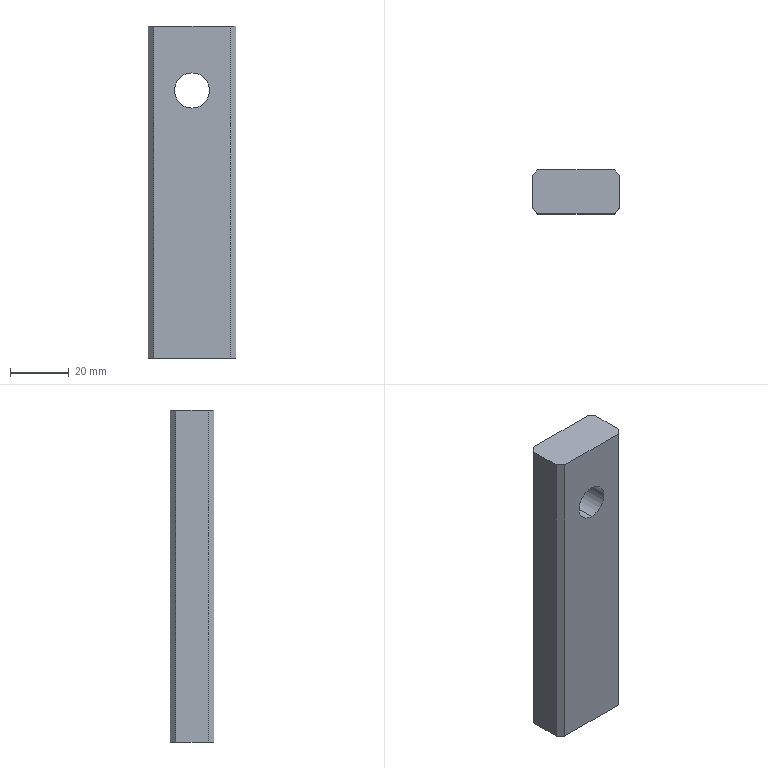Part | SolidWorks | features Cut 1, Extrusion 1, HoleWzd 1 | 1 solid | 18 faces | box 30 x 15 x 113.3 mm | volume 47736 mm3 | plane 10 | cone 4 | cylinder 4 | commonest cylinder face diameters 6.8 x2 12 x2
STEP:
#1=CARTESIAN_POINT('',(-96.6,33.5,0.625));
#2=VERTEX_POINT('',#1);
#3=CARTESIAN_POINT('',(-103.4,33.5,0.625));
#4=VERTEX_POINT('',#3);
#5=CARTESIAN_POINT('',(-100.,33.5,0.625));
#6=DIRECTION('',(0.,0.,-1.));
#7=DIRECTION('',(-1.,0.,0.));
#8=AXIS2_PLACEMENT_3D('',#5,#6,#7);
#9=CIRCLE('',#8,3.4);
#10=EDGE_CURVE('',#2,#4,#9,.T.);
#11=ORIENTED_EDGE('',*,*,#10,.F.);
#12=CARTESIAN_POINT('',(-95.975,33.5,0.));
#13=VERTEX_POINT('',#12);
#14=CARTESIAN_POINT('',(-95.975,33.5,0.));
#15=DIRECTION('',(0.7071,0.,-0.7071));
#16=VECTOR('',#15,1000.);
#17=LINE('',#14,#16);
#18=EDGE_CURVE('',#2,#13,#17,.T.);
#19=ORIENTED_EDGE('',*,*,#18,.T.);
#20=CARTESIAN_POINT('',(-104.025,33.5,0.));
#21=VERTEX_POINT('',#20);
#22=CARTESIAN_POINT('',(-100.,33.5,0.));
#23=DIRECTION('',(0.,0.,-1.));
#24=DIRECTION('',(-1.,0.,0.));
#25=AXIS2_PLACEMENT_3D('',#22,#23,#24);
#26=CIRCLE('',#25,4.025);
#27=EDGE_CURVE('',#13,#21,#26,.T.);
#28=ORIENTED_EDGE('',*,*,#27,.T.);
#29=CARTESIAN_POINT('',(-104.025,33.5,0.));
#30=DIRECTION('',(-0.7071,0.,-0.7071));
#31=VECTOR('',#30,1000.);
#32=LINE('',#29,#31);
#33=EDGE_CURVE('',#4,#21,#32,.T.);
#34=ORIENTED_EDGE('',*,*,#33,.F.);
#35=EDGE_LOOP('',(#11,#19,#28,#34));
#36=FACE_OUTER_BOUND('',#35,.T.);
#37=CARTESIAN_POINT('',(-100.,33.5,0.));
#38=DIRECTION('',(0.,0.,-1.));
#39=DIRECTION('',(-1.,0.,0.));
#40=AXIS2_PLACEMENT_3D('',#37,#38,#39);
#41=CONICAL_SURFACE('',#40,4.025,0.7854);
#42=ADVANCED_FACE('',(#36),#41,.F.);
#43=CARTESIAN_POINT('',(-96.6,33.5,17.));
#44=VERTEX_POINT('',#43);
#45=CARTESIAN_POINT('',(-103.4,33.5,17.));
#46=VERTEX_POINT('',#45);
#47=CARTESIAN_POINT('',(-100.,33.5,17.));
#48=DIRECTION('',(0.,0.,-1.));
#49=DIRECTION('',(-1.,0.,0.));
#50=AXIS2_PLACEMENT_3D('',#47,#48,#49);
#51=CIRCLE('',#50,3.4);
#52=EDGE_CURVE('',#44,#46,#51,.T.);
#53=ORIENTED_EDGE('',*,*,#52,.F.);
#54=CARTESIAN_POINT('',(-96.6,33.5,0.));
#55=DIRECTION('',(0.,0.,-1.));
#56=VECTOR('',#55,1000.);
#57=LINE('',#54,#56);
#58=EDGE_CURVE('',#44,#2,#57,.T.);
#59=ORIENTED_EDGE('',*,*,#58,.T.);
#60=ORIENTED_EDGE('',*,*,#10,.T.);
#61=CARTESIAN_POINT('',(-103.4,33.5,0.));
#62=DIRECTION('',(0.,0.,-1.));
#63=VECTOR('',#62,1000.);
#64=LINE('',#61,#63);
#65=EDGE_CURVE('',#46,#4,#64,.T.);
#66=ORIENTED_EDGE('',*,*,#65,.F.);
#67=EDGE_LOOP('',(#53,#59,#60,#66));
#68=FACE_OUTER_BOUND('',#67,.T.);
#69=CARTESIAN_POINT('',(-100.,33.5,0.));
#70=DIRECTION('',(0.,0.,-1.));
#71=DIRECTION('',(-1.,0.,0.));
#72=AXIS2_PLACEMENT_3D('',#69,#70,#71);
#73=CYLINDRICAL_SURFACE('',#72,3.4);
#74=ADVANCED_FACE('',(#68),#73,.F.);
#75=CARTESIAN_POINT('',(-100.,33.5,19.043));
#76=VERTEX_POINT('',#75);
#77=CARTESIAN_POINT('',(-103.4,33.5,17.));
#78=DIRECTION('',(-0.8572,0.,-0.515));
#79=VECTOR('',#78,1000.);
#80=LINE('',#77,#79);
#81=EDGE_CURVE('',#76,#46,#80,.T.);
#82=ORIENTED_EDGE('',*,*,#81,.F.);
#83=CARTESIAN_POINT('',(-96.6,33.5,17.));
#84=DIRECTION('',(0.8572,0.,-0.515));
#85=VECTOR('',#84,1000.);
#86=LINE('',#83,#85);
#87=EDGE_CURVE('',#76,#44,#86,.T.);
#88=ORIENTED_EDGE('',*,*,#87,.T.);
#89=ORIENTED_EDGE('',*,*,#52,.T.);
#90=EDGE_LOOP('',(#82,#88,#89));
#91=FACE_OUTER_BOUND('',#90,.T.);
#92=CARTESIAN_POINT('',(-100.,33.5,17.));
#93=DIRECTION('',(0.,0.,-1.));
#94=DIRECTION('',(-1.,0.,0.));
#95=AXIS2_PLACEMENT_3D('',#92,#93,#94);
#96=CONICAL_SURFACE('',#95,3.4,1.03);
#97=ADVANCED_FACE('',(#91),#96,.F.);
#98=CARTESIAN_POINT('',(-100.,41.,97.3));
#99=VERTEX_POINT('',#98);
#100=CARTESIAN_POINT('',(-100.,41.,85.3));
#101=VERTEX_POINT('',#100);
#102=CARTESIAN_POINT('',(-100.,41.,91.3));
#103=DIRECTION('',(0.,-1.,0.));
#104=DIRECTION('',(1.,0.,0.));
#105=AXIS2_PLACEMENT_3D('',#102,#103,#104);
#106=CIRCLE('',#105,6.);
#107=EDGE_CURVE('',#99,#101,#106,.T.);
#108=ORIENTED_EDGE('',*,*,#107,.F.);
#109=CARTESIAN_POINT('',(-100.,26.,97.3));
#110=VERTEX_POINT('',#109);
#111=CARTESIAN_POINT('',(-100.,136.,97.3));
#112=DIRECTION('',(0.,-1.,0.));
#113=VECTOR('',#112,1000.);
#114=LINE('',#111,#113);
#115=EDGE_CURVE('',#99,#110,#114,.T.);
#116=ORIENTED_EDGE('',*,*,#115,.T.);
#117=CARTESIAN_POINT('',(-100.,26.,85.3));
#118=VERTEX_POINT('',#117);
#119=CARTESIAN_POINT('',(-100.,26.,91.3));
#120=DIRECTION('',(0.,-1.,0.));
#121=DIRECTION('',(0.,0.,-1.));
#122=AXIS2_PLACEMENT_3D('',#119,#120,#121);
#123=CIRCLE('',#122,6.);
#124=EDGE_CURVE('',#110,#118,#123,.T.);
#125=ORIENTED_EDGE('',*,*,#124,.T.);
#126=CARTESIAN_POINT('',(-100.,136.,85.3));
#127=DIRECTION('',(0.,-1.,0.));
#128=VECTOR('',#127,1000.);
#129=LINE('',#126,#128);
#130=EDGE_CURVE('',#101,#118,#129,.T.);
#131=ORIENTED_EDGE('',*,*,#130,.F.);
#132=EDGE_LOOP('',(#108,#116,#125,#131));
#133=FACE_OUTER_BOUND('',#132,.T.);
#134=CARTESIAN_POINT('',(-100.,136.,91.3));
#135=DIRECTION('',(0.,-1.,0.));
#136=DIRECTION('',(0.,0.,-1.));
#137=AXIS2_PLACEMENT_3D('',#134,#135,#136);
#138=CYLINDRICAL_SURFACE('',#137,6.);
#139=ADVANCED_FACE('',(#133),#138,.F.);
#140=CARTESIAN_POINT('',(-113.,41.,0.));
#141=VERTEX_POINT('',#140);
#142=CARTESIAN_POINT('',(-115.,39.,0.));
#143=VERTEX_POINT('',#142);
#144=CARTESIAN_POINT('',(-115.,39.,0.));
#145=DIRECTION('',(-0.7071,-0.7071,0.));
#146=VECTOR('',#145,1000.);
#147=LINE('',#144,#146);
#148=EDGE_CURVE('',#141,#143,#147,.T.);
#149=ORIENTED_EDGE('',*,*,#148,.T.);
#150=CARTESIAN_POINT('',(-115.,39.,113.3));
#151=VERTEX_POINT('',#150);
#152=CARTESIAN_POINT('',(-115.,39.,113.3));
#153=DIRECTION('',(0.,0.,-1.));
#154=VECTOR('',#153,1000.);
#155=LINE('',#152,#154);
#156=EDGE_CURVE('',#151,#143,#155,.T.);
#157=ORIENTED_EDGE('',*,*,#156,.F.);
#158=CARTESIAN_POINT('',(-113.,41.,113.3));
#159=VERTEX_POINT('',#158);
#160=CARTESIAN_POINT('',(-115.,39.,113.3));
#161=DIRECTION('',(-0.7071,-0.7071,0.));
#162=VECTOR('',#161,1000.);
#163=LINE('',#160,#162);
#164=EDGE_CURVE('',#159,#151,#163,.T.);
#165=ORIENTED_EDGE('',*,*,#164,.F.);
#166=CARTESIAN_POINT('',(-113.,41.,113.3));
#167=DIRECTION('',(0.,0.,-1.));
#168=VECTOR('',#167,1000.);
#169=LINE('',#166,#168);
#170=EDGE_CURVE('',#159,#141,#169,.T.);
#171=ORIENTED_EDGE('',*,*,#170,.T.);
#172=EDGE_LOOP('',(#149,#157,#165,#171));
#173=FACE_OUTER_BOUND('',#172,.T.);
#174=CARTESIAN_POINT('',(-115.,39.,113.3));
#175=DIRECTION('',(0.7071,-0.7071,0.));
#176=DIRECTION('',(0.7071,0.7071,0.));
#177=AXIS2_PLACEMENT_3D('',#174,#175,#176);
#178=PLANE('',#177);
#179=ADVANCED_FACE('',(#173),#178,.F.);
#180=CARTESIAN_POINT('',(-115.,28.,0.));
#181=VERTEX_POINT('',#180);
#182=CARTESIAN_POINT('',(-115.,39.,0.));
#183=DIRECTION('',(0.,-1.,0.));
#184=VECTOR('',#183,1000.);
#185=LINE('',#182,#184);
#186=EDGE_CURVE('',#143,#181,#185,.T.);
#187=ORIENTED_EDGE('',*,*,#186,.T.);
#188=CARTESIAN_POINT('',(-115.,28.,113.3));
#189=VERTEX_POINT('',#188);
#190=CARTESIAN_POINT('',(-115.,28.,113.3));
#191=DIRECTION('',(0.,0.,-1.));
#192=VECTOR('',#191,1000.);
#193=LINE('',#190,#192);
#194=EDGE_CURVE('',#189,#181,#193,.T.);
#195=ORIENTED_EDGE('',*,*,#194,.F.);
#196=CARTESIAN_POINT('',(-115.,39.,113.3));
#197=DIRECTION('',(0.,-1.,0.));
#198=VECTOR('',#197,1000.);
#199=LINE('',#196,#198);
#200=EDGE_CURVE('',#151,#189,#199,.T.);
#201=ORIENTED_EDGE('',*,*,#200,.F.);
#202=ORIENTED_EDGE('',*,*,#156,.T.);
#203=EDGE_LOOP('',(#187,#195,#201,#202));
#204=FACE_OUTER_BOUND('',#203,.T.);
#205=CARTESIAN_POINT('',(-115.,39.,113.3));
#206=DIRECTION('',(1.,0.,0.));
#207=DIRECTION('',(0.,0.,-1.));
#208=AXIS2_PLACEMENT_3D('',#205,#206,#207);
#209=PLANE('',#208);
#210=ADVANCED_FACE('',(#204),#209,.F.);
#211=CARTESIAN_POINT('',(-113.,26.,0.));
#212=VERTEX_POINT('',#211);
#213=CARTESIAN_POINT('',(-115.,28.,0.));
#214=DIRECTION('',(0.7071,-0.7071,0.));
#215=VECTOR('',#214,1000.);
#216=LINE('',#213,#215);
#217=EDGE_CURVE('',#181,#212,#216,.T.);
#218=ORIENTED_EDGE('',*,*,#217,.T.);
#219=CARTESIAN_POINT('',(-113.,26.,113.3));
#220=VERTEX_POINT('',#219);
#221=CARTESIAN_POINT('',(-113.,26.,113.3));
#222=DIRECTION('',(0.,0.,-1.));
#223=VECTOR('',#222,1000.);
#224=LINE('',#221,#223);
#225=EDGE_CURVE('',#220,#212,#224,.T.);
#226=ORIENTED_EDGE('',*,*,#225,.F.);
#227=CARTESIAN_POINT('',(-115.,28.,113.3));
#228=DIRECTION('',(0.7071,-0.7071,0.));
#229=VECTOR('',#228,1000.);
#230=LINE('',#227,#229);
#231=EDGE_CURVE('',#189,#220,#230,.T.);
#232=ORIENTED_EDGE('',*,*,#231,.F.);
#233=ORIENTED_EDGE('',*,*,#194,.T.);
#234=EDGE_LOOP('',(#218,#226,#232,#233));
#235=FACE_OUTER_BOUND('',#234,.T.);
#236=CARTESIAN_POINT('',(-115.,28.,113.3));
#237=DIRECTION('',(0.7071,0.7071,0.));
#238=DIRECTION('',(-0.7071,0.7071,0.));
#239=AXIS2_PLACEMENT_3D('',#236,#237,#238);
#240=PLANE('',#239);
#241=ADVANCED_FACE('',(#235),#240,.F.);
#242=CARTESIAN_POINT('',(-100.,26.,91.3));
#243=DIRECTION('',(0.,-1.,0.));
#244=DIRECTION('',(0.,0.,-1.));
#245=AXIS2_PLACEMENT_3D('',#242,#243,#244);
#246=CIRCLE('',#245,6.);
#247=EDGE_CURVE('',#118,#110,#246,.T.);
#248=ORIENTED_EDGE('',*,*,#247,.F.);
#249=ORIENTED_EDGE('',*,*,#124,.F.);
#250=EDGE_LOOP('',(#248,#249));
#251=FACE_BOUND('',#250,.T.);
#252=CARTESIAN_POINT('',(-87.,26.,0.));
#253=VERTEX_POINT('',#252);
#254=CARTESIAN_POINT('',(-113.,26.,0.));
#255=DIRECTION('',(1.,0.,0.));
#256=VECTOR('',#255,1000.);
#257=LINE('',#254,#256);
#258=EDGE_CURVE('',#212,#253,#257,.T.);
#259=ORIENTED_EDGE('',*,*,#258,.T.);
#260=CARTESIAN_POINT('',(-87.,26.,113.3));
#261=VERTEX_POINT('',#260);
#262=CARTESIAN_POINT('',(-87.,26.,113.3));
#263=DIRECTION('',(0.,0.,-1.));
#264=VECTOR('',#263,1000.);
#265=LINE('',#262,#264);
#266=EDGE_CURVE('',#261,#253,#265,.T.);
#267=ORIENTED_EDGE('',*,*,#266,.F.);
#268=CARTESIAN_POINT('',(-113.,26.,113.3));
#269=DIRECTION('',(1.,0.,0.));
#270=VECTOR('',#269,1000.);
#271=LINE('',#268,#270);
#272=EDGE_CURVE('',#220,#261,#271,.T.);
#273=ORIENTED_EDGE('',*,*,#272,.F.);
#274=ORIENTED_EDGE('',*,*,#225,.T.);
#275=EDGE_LOOP('',(#259,#267,#273,#274));
#276=FACE_OUTER_BOUND('',#275,.T.);
#277=CARTESIAN_POINT('',(-113.,26.,113.3));
#278=DIRECTION('',(0.,1.,0.));
#279=DIRECTION('',(0.,0.,1.));
#280=AXIS2_PLACEMENT_3D('',#277,#278,#279);
#281=PLANE('',#280);
#282=ADVANCED_FACE('',(#251,#276),#281,.F.);
#283=CARTESIAN_POINT('',(-85.,28.,0.));
#284=VERTEX_POINT('',#283);
#285=CARTESIAN_POINT('',(-85.,28.,0.));
#286=DIRECTION('',(0.7071,0.7071,0.));
#287=VECTOR('',#286,1000.);
#288=LINE('',#285,#287);
#289=EDGE_CURVE('',#253,#284,#288,.T.);
#290=ORIENTED_EDGE('',*,*,#289,.T.);
#291=CARTESIAN_POINT('',(-85.,28.,113.3));
#292=VERTEX_POINT('',#291);
#293=CARTESIAN_POINT('',(-85.,28.,113.3));
#294=DIRECTION('',(0.,0.,-1.));
#295=VECTOR('',#294,1000.);
#296=LINE('',#293,#295);
#297=EDGE_CURVE('',#292,#284,#296,.T.);
#298=ORIENTED_EDGE('',*,*,#297,.F.);
#299=CARTESIAN_POINT('',(-85.,28.,113.3));
#300=DIRECTION('',(0.7071,0.7071,0.));
#301=VECTOR('',#300,1000.);
#302=LINE('',#299,#301);
#303=EDGE_CURVE('',#261,#292,#302,.T.);
#304=ORIENTED_EDGE('',*,*,#303,.F.);
#305=ORIENTED_EDGE('',*,*,#266,.T.);
#306=EDGE_LOOP('',(#290,#298,#304,#305));
#307=FACE_OUTER_BOUND('',#306,.T.);
#308=CARTESIAN_POINT('',(-85.,28.,113.3));
#309=DIRECTION('',(-0.7071,0.7071,0.));
#310=DIRECTION('',(-0.7071,-0.7071,0.));
#311=AXIS2_PLACEMENT_3D('',#308,#309,#310);
#312=PLANE('',#311);
#313=ADVANCED_FACE('',(#307),#312,.F.);
#314=CARTESIAN_POINT('',(-85.,39.,0.));
#315=VERTEX_POINT('',#314);
#316=CARTESIAN_POINT('',(-85.,39.,0.));
#317=DIRECTION('',(0.,1.,0.));
#318=VECTOR('',#317,1000.);
#319=LINE('',#316,#318);
#320=EDGE_CURVE('',#284,#315,#319,.T.);
#321=ORIENTED_EDGE('',*,*,#320,.T.);
#322=CARTESIAN_POINT('',(-85.,39.,113.3));
#323=VERTEX_POINT('',#322);
#324=CARTESIAN_POINT('',(-85.,39.,113.3));
#325=DIRECTION('',(0.,0.,-1.));
#326=VECTOR('',#325,1000.);
#327=LINE('',#324,#326);
#328=EDGE_CURVE('',#323,#315,#327,.T.);
#329=ORIENTED_EDGE('',*,*,#328,.F.);
#330=CARTESIAN_POINT('',(-85.,39.,113.3));
#331=DIRECTION('',(0.,1.,0.));
#332=VECTOR('',#331,1000.);
#333=LINE('',#330,#332);
#334=EDGE_CURVE('',#292,#323,#333,.T.);
#335=ORIENTED_EDGE('',*,*,#334,.F.);
#336=ORIENTED_EDGE('',*,*,#297,.T.);
#337=EDGE_LOOP('',(#321,#329,#335,#336));
#338=FACE_OUTER_BOUND('',#337,.T.);
#339=CARTESIAN_POINT('',(-85.,39.,113.3));
#340=DIRECTION('',(-1.,0.,0.));
#341=DIRECTION('',(0.,-1.,0.));
#342=AXIS2_PLACEMENT_3D('',#339,#340,#341);
#343=PLANE('',#342);
#344=ADVANCED_FACE('',(#338),#343,.F.);
#345=CARTESIAN_POINT('',(-87.,41.,0.));
#346=VERTEX_POINT('',#345);
#347=CARTESIAN_POINT('',(-87.,41.,0.));
#348=DIRECTION('',(-0.7071,0.7071,0.));
#349=VECTOR('',#348,1000.);
#350=LINE('',#347,#349);
#351=EDGE_CURVE('',#315,#346,#350,.T.);
#352=ORIENTED_EDGE('',*,*,#351,.T.);
#353=CARTESIAN_POINT('',(-87.,41.,113.3));
#354=VERTEX_POINT('',#353);
#355=CARTESIAN_POINT('',(-87.,41.,113.3));
#356=DIRECTION('',(0.,0.,-1.));
#357=VECTOR('',#356,1000.);
#358=LINE('',#355,#357);
#359=EDGE_CURVE('',#354,#346,#358,.T.);
#360=ORIENTED_EDGE('',*,*,#359,.F.);
#361=CARTESIAN_POINT('',(-87.,41.,113.3));
#362=DIRECTION('',(-0.7071,0.7071,0.));
#363=VECTOR('',#362,1000.);
#364=LINE('',#361,#363);
#365=EDGE_CURVE('',#323,#354,#364,.T.);
#366=ORIENTED_EDGE('',*,*,#365,.F.);
#367=ORIENTED_EDGE('',*,*,#328,.T.);
#368=EDGE_LOOP('',(#352,#360,#366,#367));
#369=FACE_OUTER_BOUND('',#368,.T.);
#370=CARTESIAN_POINT('',(-87.,41.,113.3));
#371=DIRECTION('',(-0.7071,-0.7071,0.));
#372=DIRECTION('',(0.7071,-0.7071,0.));
#373=AXIS2_PLACEMENT_3D('',#370,#371,#372);
#374=PLANE('',#373);
#375=ADVANCED_FACE('',(#369),#374,.F.);
#376=CARTESIAN_POINT('',(-100.,41.,91.3));
#377=DIRECTION('',(0.,-1.,0.));
#378=DIRECTION('',(1.,0.,0.));
#379=AXIS2_PLACEMENT_3D('',#376,#377,#378);
#380=CIRCLE('',#379,6.);
#381=EDGE_CURVE('',#101,#99,#380,.T.);
#382=ORIENTED_EDGE('',*,*,#381,.T.);
#383=ORIENTED_EDGE('',*,*,#107,.T.);
#384=EDGE_LOOP('',(#382,#383));
#385=FACE_BOUND('',#384,.T.);
#386=CARTESIAN_POINT('',(-113.,41.,0.));
#387=DIRECTION('',(-1.,0.,0.));
#388=VECTOR('',#387,1000.);
#389=LINE('',#386,#388);
#390=EDGE_CURVE('',#346,#141,#389,.T.);
#391=ORIENTED_EDGE('',*,*,#390,.T.);
#392=ORIENTED_EDGE('',*,*,#170,.F.);
#393=CARTESIAN_POINT('',(-113.,41.,113.3));
#394=DIRECTION('',(-1.,0.,0.));
#395=VECTOR('',#394,1000.);
#396=LINE('',#393,#395);
#397=EDGE_CURVE('',#354,#159,#396,.T.);
#398=ORIENTED_EDGE('',*,*,#397,.F.);
#399=ORIENTED_EDGE('',*,*,#359,.T.);
#400=EDGE_LOOP('',(#391,#392,#398,#399));
#401=FACE_OUTER_BOUND('',#400,.T.);
#402=CARTESIAN_POINT('',(-113.,41.,113.3));
#403=DIRECTION('',(0.,-1.,0.));
#404=DIRECTION('',(1.,0.,0.));
#405=AXIS2_PLACEMENT_3D('',#402,#403,#404);
#406=PLANE('',#405);
#407=ADVANCED_FACE('',(#385,#401),#406,.F.);
#408=ORIENTED_EDGE('',*,*,#164,.T.);
#409=ORIENTED_EDGE('',*,*,#200,.T.);
#410=ORIENTED_EDGE('',*,*,#231,.T.);
#411=ORIENTED_EDGE('',*,*,#272,.T.);
#412=ORIENTED_EDGE('',*,*,#303,.T.);
#413=ORIENTED_EDGE('',*,*,#334,.T.);
#414=ORIENTED_EDGE('',*,*,#365,.T.);
#415=ORIENTED_EDGE('',*,*,#397,.T.);
#416=EDGE_LOOP('',(#408,#409,#410,#411,#412,#413,#414,#415));
#417=FACE_OUTER_BOUND('',#416,.T.);
#418=CARTESIAN_POINT('',(0.,0.,113.3));
#419=DIRECTION('',(0.,0.,-1.));
#420=DIRECTION('',(-1.,0.,0.));
#421=AXIS2_PLACEMENT_3D('',#418,#419,#420);
#422=PLANE('',#421);
#423=ADVANCED_FACE('',(#417),#422,.F.);
#424=CARTESIAN_POINT('',(-100.,33.5,0.));
#425=DIRECTION('',(0.,0.,-1.));
#426=DIRECTION('',(-1.,0.,0.));
#427=AXIS2_PLACEMENT_3D('',#424,#425,#426);
#428=CIRCLE('',#427,4.025);
#429=EDGE_CURVE('',#21,#13,#428,.T.);
#430=ORIENTED_EDGE('',*,*,#429,.F.);
#431=ORIENTED_EDGE('',*,*,#27,.F.);
#432=EDGE_LOOP('',(#430,#431));
#433=FACE_BOUND('',#432,.T.);
#434=ORIENTED_EDGE('',*,*,#148,.F.);
#435=ORIENTED_EDGE('',*,*,#390,.F.);
#436=ORIENTED_EDGE('',*,*,#351,.F.);
#437=ORIENTED_EDGE('',*,*,#320,.F.);
#438=ORIENTED_EDGE('',*,*,#289,.F.);
#439=ORIENTED_EDGE('',*,*,#258,.F.);
#440=ORIENTED_EDGE('',*,*,#217,.F.);
#441=ORIENTED_EDGE('',*,*,#186,.F.);
#442=EDGE_LOOP('',(#434,#435,#436,#437,#438,#439,#440,#441));
#443=FACE_OUTER_BOUND('',#442,.T.);
#444=CARTESIAN_POINT('',(0.,0.,0.));
#445=DIRECTION('',(0.,0.,-1.));
#446=DIRECTION('',(-1.,0.,0.));
#447=AXIS2_PLACEMENT_3D('',#444,#445,#446);
#448=PLANE('',#447);
#449=ADVANCED_FACE('',(#433,#443),#448,.T.);
#450=ORIENTED_EDGE('',*,*,#115,.F.);
#451=ORIENTED_EDGE('',*,*,#381,.F.);
#452=ORIENTED_EDGE('',*,*,#130,.T.);
#453=ORIENTED_EDGE('',*,*,#247,.T.);
#454=EDGE_LOOP('',(#450,#451,#452,#453));
#455=FACE_OUTER_BOUND('',#454,.T.);
#456=CARTESIAN_POINT('',(-100.,136.,91.3));
#457=DIRECTION('',(0.,-1.,0.));
#458=DIRECTION('',(0.,0.,-1.));
#459=AXIS2_PLACEMENT_3D('',#456,#457,#458);
#460=CYLINDRICAL_SURFACE('',#459,6.);
#461=ADVANCED_FACE('',(#455),#460,.F.);
#462=ORIENTED_EDGE('',*,*,#87,.F.);
#463=ORIENTED_EDGE('',*,*,#81,.T.);
#464=CARTESIAN_POINT('',(-100.,33.5,17.));
#465=DIRECTION('',(0.,0.,-1.));
#466=DIRECTION('',(-1.,0.,0.));
#467=AXIS2_PLACEMENT_3D('',#464,#465,#466);
#468=CIRCLE('',#467,3.4);
#469=EDGE_CURVE('',#46,#44,#468,.T.);
#470=ORIENTED_EDGE('',*,*,#469,.T.);
#471=EDGE_LOOP('',(#462,#463,#470));
#472=FACE_OUTER_BOUND('',#471,.T.);
#473=CARTESIAN_POINT('',(-100.,33.5,17.));
#474=DIRECTION('',(0.,0.,-1.));
#475=DIRECTION('',(-1.,0.,0.));
#476=AXIS2_PLACEMENT_3D('',#473,#474,#475);
#477=CONICAL_SURFACE('',#476,3.4,1.03);
#478=ADVANCED_FACE('',(#472),#477,.F.);
#479=ORIENTED_EDGE('',*,*,#58,.F.);
#480=ORIENTED_EDGE('',*,*,#469,.F.);
#481=ORIENTED_EDGE('',*,*,#65,.T.);
#482=CARTESIAN_POINT('',(-100.,33.5,0.625));
#483=DIRECTION('',(0.,0.,-1.));
#484=DIRECTION('',(-1.,0.,0.));
#485=AXIS2_PLACEMENT_3D('',#482,#483,#484);
#486=CIRCLE('',#485,3.4);
#487=EDGE_CURVE('',#4,#2,#486,.T.);
#488=ORIENTED_EDGE('',*,*,#487,.T.);
#489=EDGE_LOOP('',(#479,#480,#481,#488));
#490=FACE_OUTER_BOUND('',#489,.T.);
#491=CARTESIAN_POINT('',(-100.,33.5,0.));
#492=DIRECTION('',(0.,0.,-1.));
#493=DIRECTION('',(-1.,0.,0.));
#494=AXIS2_PLACEMENT_3D('',#491,#492,#493);
#495=CYLINDRICAL_SURFACE('',#494,3.4);
#496=ADVANCED_FACE('',(#490),#495,.F.);
#497=ORIENTED_EDGE('',*,*,#18,.F.);
#498=ORIENTED_EDGE('',*,*,#487,.F.);
#499=ORIENTED_EDGE('',*,*,#33,.T.);
#500=ORIENTED_EDGE('',*,*,#429,.T.);
#501=EDGE_LOOP('',(#497,#498,#499,#500));
#502=FACE_OUTER_BOUND('',#501,.T.);
#503=CARTESIAN_POINT('',(-100.,33.5,0.));
#504=DIRECTION('',(0.,0.,-1.));
#505=DIRECTION('',(-1.,0.,0.));
#506=AXIS2_PLACEMENT_3D('',#503,#504,#505);
#507=CONICAL_SURFACE('',#506,4.025,0.7854);
#508=ADVANCED_FACE('',(#502),#507,.F.);
#509=CLOSED_SHELL('',(#42,#74,#97,#139,#179,#210,#241,#282,#313,#344,#375,#407,#423,#449,#461,#478,#496,#508));
#510=MANIFOLD_SOLID_BREP('',#509);
#511=CARTESIAN_POINT('',(0.,0.,0.));
#512=DIRECTION('',(0.,0.,1.));
#513=DIRECTION('',(1.,0.,0.));
#514=AXIS2_PLACEMENT_3D('',#511,#512,#513);
#515=(LENGTH_UNIT()NAMED_UNIT(*)SI_UNIT(.MILLI.,.METRE.));
#516=UNCERTAINTY_MEASURE_WITH_UNIT(LENGTH_MEASURE(0.00001),#515,'','');
#517=(NAMED_UNIT(*)PLANE_ANGLE_UNIT()SI_UNIT($,.RADIAN.));
#518=(NAMED_UNIT(*)SI_UNIT($,.STERADIAN.)SOLID_ANGLE_UNIT());
#519=(GEOMETRIC_REPRESENTATION_CONTEXT(3)GLOBAL_UNCERTAINTY_ASSIGNED_CONTEXT((#516))GLOBAL_UNIT_ASSIGNED_CONTEXT((#515,#517,#518))REPRESENTATION_CONTEXT('',''));
#520=ADVANCED_BREP_SHAPE_REPRESENTATION('',(#510,#514),#519);